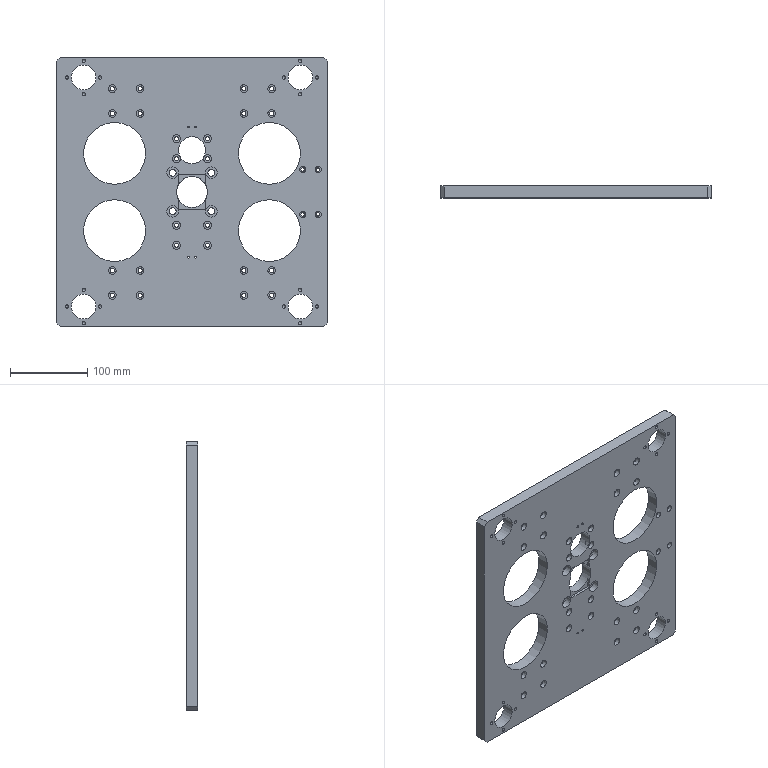Part | NX | 1 solid | 164 faces | box 350 x 15 x 348 mm | volume 1413615 mm3 | cylinder 98 | plane 50 | cone 16 | commonest cylinder face diameters 5.5 x24 10 x24 4.2 x16 2.5 x4 4 x4 4.5 x4